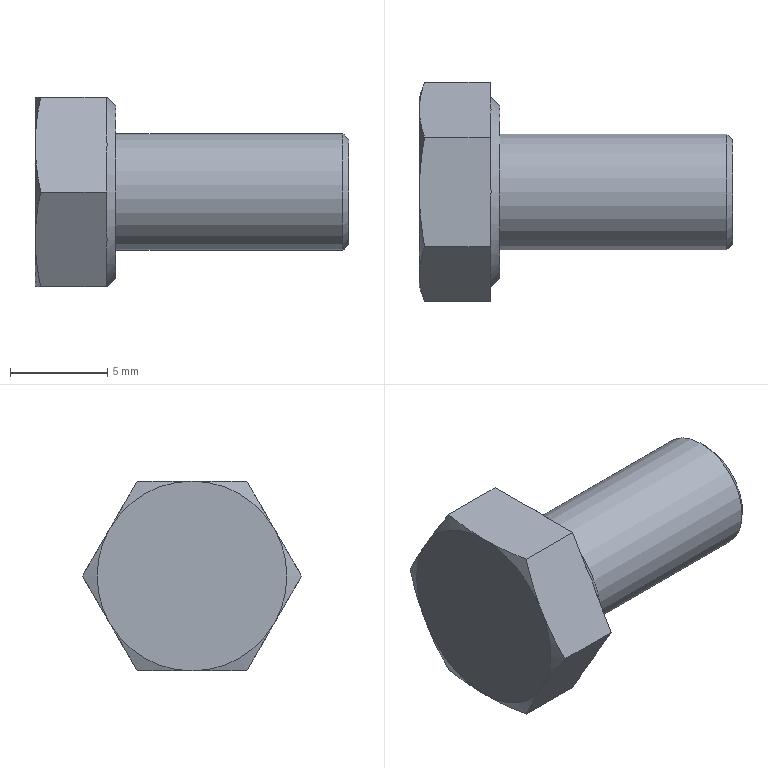Part | STEP file | hexagon head bolts-full thread gb_GB_FASTENER_BOLT_STBAB A M6X12-C | 1 solid | 24 faces | box 16.15 x 11.293 x 9.78 mm | volume 674.74 mm3 | plane 15 | cone 8 | cylinder 1 | commonest cylinder face diameters 6 x1